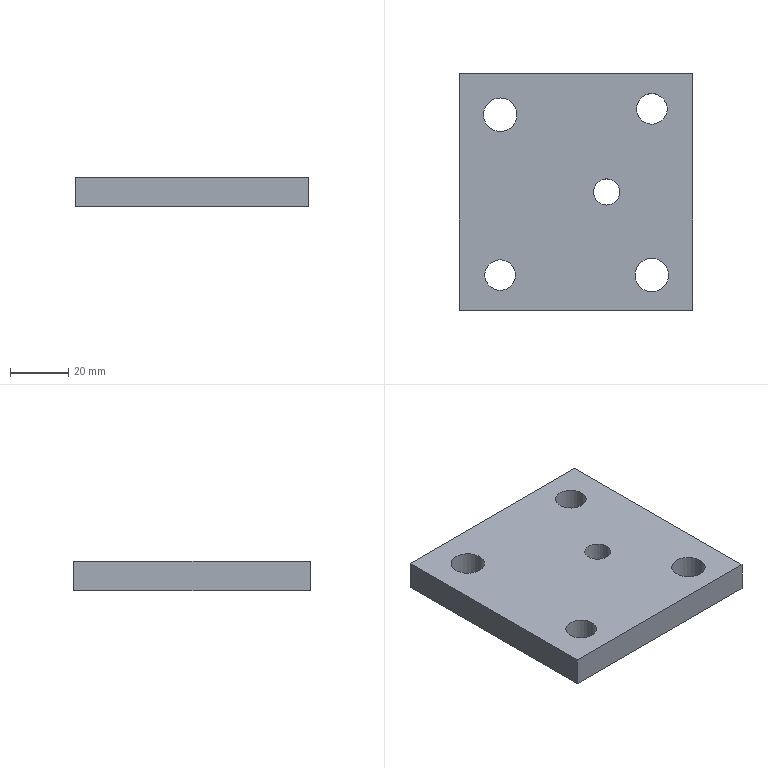Part | NX | features 6 2 | 1 solid | 11 faces | box 80 x 81 x 10 mm | volume 60355 mm3 | plane 6 | cylinder 5 | commonest cylinder face diameters 10.5 x2 11.5 x2 9 x1
STEP:
#1=CARTESIAN_POINT('',(3424.438,82.438,101.));
#2=VERTEX_POINT('',#1);
#3=CARTESIAN_POINT('',(3424.438,1.438,101.));
#4=VERTEX_POINT('',#3);
#5=CARTESIAN_POINT('',(3424.438,41.938,101.));
#6=DIRECTION('',(0.,-1.,0.));
#7=VECTOR('',#6,1000.);
#8=LINE('',#5,#7);
#9=EDGE_CURVE('',#2,#4,#8,.T.);
#10=ORIENTED_EDGE('',*,*,#9,.T.);
#11=CARTESIAN_POINT('',(3424.438,1.438,91.));
#12=VERTEX_POINT('',#11);
#13=CARTESIAN_POINT('',(3424.438,1.438,91.));
#14=DIRECTION('',(0.,0.,1.));
#15=VECTOR('',#14,1000.);
#16=LINE('',#13,#15);
#17=EDGE_CURVE('',#12,#4,#16,.T.);
#18=ORIENTED_EDGE('',*,*,#17,.F.);
#19=CARTESIAN_POINT('',(3424.438,82.438,91.));
#20=VERTEX_POINT('',#19);
#21=CARTESIAN_POINT('',(3424.438,41.938,91.));
#22=DIRECTION('',(0.,-1.,0.));
#23=VECTOR('',#22,1000.);
#24=LINE('',#21,#23);
#25=EDGE_CURVE('',#20,#12,#24,.T.);
#26=ORIENTED_EDGE('',*,*,#25,.F.);
#27=CARTESIAN_POINT('',(3424.438,82.438,91.));
#28=DIRECTION('',(0.,0.,-1.));
#29=VECTOR('',#28,1000.);
#30=LINE('',#27,#29);
#31=EDGE_CURVE('',#2,#20,#30,.T.);
#32=ORIENTED_EDGE('',*,*,#31,.F.);
#33=EDGE_LOOP('',(#10,#18,#26,#32));
#34=FACE_BOUND('',#33,.T.);
#35=CARTESIAN_POINT('',(3424.438,41.938,91.));
#36=DIRECTION('',(-1.,0.,0.));
#37=DIRECTION('',(0.,-1.,0.));
#38=AXIS2_PLACEMENT_3D('',#35,#36,#37);
#39=PLANE('',#38);
#40=ADVANCED_FACE('',(#34),#39,.F.);
#41=CARTESIAN_POINT('',(3344.438,82.438,101.));
#42=VERTEX_POINT('',#41);
#43=CARTESIAN_POINT('',(3374.438,82.438,101.));
#44=DIRECTION('',(1.,0.,0.));
#45=VECTOR('',#44,1000.);
#46=LINE('',#43,#45);
#47=EDGE_CURVE('',#42,#2,#46,.T.);
#48=ORIENTED_EDGE('',*,*,#47,.T.);
#49=ORIENTED_EDGE('',*,*,#31,.T.);
#50=CARTESIAN_POINT('',(3344.438,82.438,91.));
#51=VERTEX_POINT('',#50);
#52=CARTESIAN_POINT('',(3374.438,82.438,91.));
#53=DIRECTION('',(1.,0.,0.));
#54=VECTOR('',#53,1000.);
#55=LINE('',#52,#54);
#56=EDGE_CURVE('',#51,#20,#55,.T.);
#57=ORIENTED_EDGE('',*,*,#56,.F.);
#58=CARTESIAN_POINT('',(3344.438,82.438,91.));
#59=DIRECTION('',(0.,0.,-1.));
#60=VECTOR('',#59,1000.);
#61=LINE('',#58,#60);
#62=EDGE_CURVE('',#42,#51,#61,.T.);
#63=ORIENTED_EDGE('',*,*,#62,.F.);
#64=EDGE_LOOP('',(#48,#49,#57,#63));
#65=FACE_BOUND('',#64,.T.);
#66=CARTESIAN_POINT('',(3374.438,82.438,91.));
#67=DIRECTION('',(0.,-1.,0.));
#68=DIRECTION('',(1.,0.,0.));
#69=AXIS2_PLACEMENT_3D('',#66,#67,#68);
#70=PLANE('',#69);
#71=ADVANCED_FACE('',(#65),#70,.F.);
#72=CARTESIAN_POINT('',(3344.438,1.438,101.));
#73=VERTEX_POINT('',#72);
#74=CARTESIAN_POINT('',(3344.438,41.938,101.));
#75=DIRECTION('',(0.,1.,0.));
#76=VECTOR('',#75,1000.);
#77=LINE('',#74,#76);
#78=EDGE_CURVE('',#73,#42,#77,.T.);
#79=ORIENTED_EDGE('',*,*,#78,.T.);
#80=ORIENTED_EDGE('',*,*,#62,.T.);
#81=CARTESIAN_POINT('',(3344.438,1.438,91.));
#82=VERTEX_POINT('',#81);
#83=CARTESIAN_POINT('',(3344.438,41.938,91.));
#84=DIRECTION('',(0.,1.,0.));
#85=VECTOR('',#84,1000.);
#86=LINE('',#83,#85);
#87=EDGE_CURVE('',#82,#51,#86,.T.);
#88=ORIENTED_EDGE('',*,*,#87,.F.);
#89=CARTESIAN_POINT('',(3344.438,1.438,91.));
#90=DIRECTION('',(0.,0.,-1.));
#91=VECTOR('',#90,1000.);
#92=LINE('',#89,#91);
#93=EDGE_CURVE('',#73,#82,#92,.T.);
#94=ORIENTED_EDGE('',*,*,#93,.F.);
#95=EDGE_LOOP('',(#79,#80,#88,#94));
#96=FACE_BOUND('',#95,.T.);
#97=CARTESIAN_POINT('',(3344.438,41.938,91.));
#98=DIRECTION('',(1.,0.,0.));
#99=DIRECTION('',(0.,1.,0.));
#100=AXIS2_PLACEMENT_3D('',#97,#98,#99);
#101=PLANE('',#100);
#102=ADVANCED_FACE('',(#96),#101,.F.);
#103=CARTESIAN_POINT('',(3358.438,8.188,91.));
#104=VERTEX_POINT('',#103);
#105=CARTESIAN_POINT('',(3358.438,13.438,91.));
#106=DIRECTION('',(0.,0.,-1.));
#107=DIRECTION('',(0.,-1.,0.));
#108=AXIS2_PLACEMENT_3D('',#105,#106,#107);
#109=CIRCLE('',#108,5.25);
#110=EDGE_CURVE('',#104,#104,#109,.T.);
#111=ORIENTED_EDGE('',*,*,#110,.T.);
#112=EDGE_LOOP('',(#111));
#113=FACE_BOUND('',#112,.T.);
#114=CARTESIAN_POINT('',(3358.438,18.688,101.));
#115=VERTEX_POINT('',#114);
#116=CARTESIAN_POINT('',(3358.438,13.438,101.));
#117=DIRECTION('',(0.,0.,1.));
#118=DIRECTION('',(0.,1.,0.));
#119=AXIS2_PLACEMENT_3D('',#116,#117,#118);
#120=CIRCLE('',#119,5.25);
#121=EDGE_CURVE('',#115,#115,#120,.T.);
#122=ORIENTED_EDGE('',*,*,#121,.T.);
#123=EDGE_LOOP('',(#122));
#124=FACE_BOUND('',#123,.T.);
#125=CARTESIAN_POINT('',(3358.438,13.438,91.));
#126=DIRECTION('',(0.,0.,1.));
#127=DIRECTION('',(0.,-1.,0.));
#128=AXIS2_PLACEMENT_3D('',#125,#126,#127);
#129=CYLINDRICAL_SURFACE('',#128,5.25);
#130=ADVANCED_FACE('',(#113,#124),#129,.F.);
#131=CARTESIAN_POINT('',(3410.438,19.188,91.));
#132=VERTEX_POINT('',#131);
#133=CARTESIAN_POINT('',(3410.438,13.438,91.));
#134=DIRECTION('',(0.,0.,1.));
#135=DIRECTION('',(0.,1.,0.));
#136=AXIS2_PLACEMENT_3D('',#133,#134,#135);
#137=CIRCLE('',#136,5.75);
#138=EDGE_CURVE('',#132,#132,#137,.T.);
#139=ORIENTED_EDGE('',*,*,#138,.F.);
#140=EDGE_LOOP('',(#139));
#141=FACE_BOUND('',#140,.T.);
#142=CARTESIAN_POINT('',(3410.438,19.188,101.));
#143=VERTEX_POINT('',#142);
#144=CARTESIAN_POINT('',(3410.438,13.438,101.));
#145=DIRECTION('',(0.,0.,1.));
#146=DIRECTION('',(0.,1.,0.));
#147=AXIS2_PLACEMENT_3D('',#144,#145,#146);
#148=CIRCLE('',#147,5.75);
#149=EDGE_CURVE('',#143,#143,#148,.T.);
#150=ORIENTED_EDGE('',*,*,#149,.T.);
#151=EDGE_LOOP('',(#150));
#152=FACE_BOUND('',#151,.T.);
#153=CARTESIAN_POINT('',(3410.438,13.438,91.));
#154=DIRECTION('',(0.,0.,1.));
#155=DIRECTION('',(0.,-1.,0.));
#156=AXIS2_PLACEMENT_3D('',#153,#154,#155);
#157=CYLINDRICAL_SURFACE('',#156,5.75);
#158=ADVANCED_FACE('',(#141,#152),#157,.F.);
#159=CARTESIAN_POINT('',(3374.438,1.438,91.));
#160=DIRECTION('',(-1.,0.,0.));
#161=VECTOR('',#160,1000.);
#162=LINE('',#159,#161);
#163=EDGE_CURVE('',#12,#82,#162,.T.);
#164=ORIENTED_EDGE('',*,*,#163,.F.);
#165=ORIENTED_EDGE('',*,*,#17,.T.);
#166=CARTESIAN_POINT('',(3374.438,1.438,101.));
#167=DIRECTION('',(-1.,0.,0.));
#168=VECTOR('',#167,1000.);
#169=LINE('',#166,#168);
#170=EDGE_CURVE('',#4,#73,#169,.T.);
#171=ORIENTED_EDGE('',*,*,#170,.T.);
#172=ORIENTED_EDGE('',*,*,#93,.T.);
#173=EDGE_LOOP('',(#164,#165,#171,#172));
#174=FACE_BOUND('',#173,.T.);
#175=CARTESIAN_POINT('',(3374.438,1.438,91.));
#176=DIRECTION('',(0.,1.,0.));
#177=DIRECTION('',(-1.,0.,0.));
#178=AXIS2_PLACEMENT_3D('',#175,#176,#177);
#179=PLANE('',#178);
#180=ADVANCED_FACE('',(#174),#179,.F.);
#181=CARTESIAN_POINT('',(3358.438,74.188,91.));
#182=VERTEX_POINT('',#181);
#183=CARTESIAN_POINT('',(3358.438,68.438,91.));
#184=DIRECTION('',(0.,0.,1.));
#185=DIRECTION('',(0.,1.,0.));
#186=AXIS2_PLACEMENT_3D('',#183,#184,#185);
#187=CIRCLE('',#186,5.75);
#188=EDGE_CURVE('',#182,#182,#187,.T.);
#189=ORIENTED_EDGE('',*,*,#188,.F.);
#190=EDGE_LOOP('',(#189));
#191=FACE_BOUND('',#190,.T.);
#192=CARTESIAN_POINT('',(3358.438,74.188,101.));
#193=VERTEX_POINT('',#192);
#194=CARTESIAN_POINT('',(3358.438,68.438,101.));
#195=DIRECTION('',(0.,0.,1.));
#196=DIRECTION('',(0.,1.,0.));
#197=AXIS2_PLACEMENT_3D('',#194,#195,#196);
#198=CIRCLE('',#197,5.75);
#199=EDGE_CURVE('',#193,#193,#198,.T.);
#200=ORIENTED_EDGE('',*,*,#199,.T.);
#201=EDGE_LOOP('',(#200));
#202=FACE_BOUND('',#201,.T.);
#203=CARTESIAN_POINT('',(3358.438,68.438,91.));
#204=DIRECTION('',(0.,0.,1.));
#205=DIRECTION('',(0.,-1.,0.));
#206=AXIS2_PLACEMENT_3D('',#203,#204,#205);
#207=CYLINDRICAL_SURFACE('',#206,5.75);
#208=ADVANCED_FACE('',(#191,#202),#207,.F.);
#209=CARTESIAN_POINT('',(3410.438,65.188,91.));
#210=VERTEX_POINT('',#209);
#211=CARTESIAN_POINT('',(3410.438,70.438,91.));
#212=DIRECTION('',(0.,0.,-1.));
#213=DIRECTION('',(0.,-1.,0.));
#214=AXIS2_PLACEMENT_3D('',#211,#212,#213);
#215=CIRCLE('',#214,5.25);
#216=EDGE_CURVE('',#210,#210,#215,.T.);
#217=ORIENTED_EDGE('',*,*,#216,.T.);
#218=EDGE_LOOP('',(#217));
#219=FACE_BOUND('',#218,.T.);
#220=CARTESIAN_POINT('',(3410.438,75.688,101.));
#221=VERTEX_POINT('',#220);
#222=CARTESIAN_POINT('',(3410.438,70.438,101.));
#223=DIRECTION('',(0.,0.,1.));
#224=DIRECTION('',(0.,1.,0.));
#225=AXIS2_PLACEMENT_3D('',#222,#223,#224);
#226=CIRCLE('',#225,5.25);
#227=EDGE_CURVE('',#221,#221,#226,.T.);
#228=ORIENTED_EDGE('',*,*,#227,.T.);
#229=EDGE_LOOP('',(#228));
#230=FACE_BOUND('',#229,.T.);
#231=CARTESIAN_POINT('',(3410.438,70.438,91.));
#232=DIRECTION('',(0.,0.,1.));
#233=DIRECTION('',(0.,-1.,0.));
#234=AXIS2_PLACEMENT_3D('',#231,#232,#233);
#235=CYLINDRICAL_SURFACE('',#234,5.25);
#236=ADVANCED_FACE('',(#219,#230),#235,.F.);
#237=CARTESIAN_POINT('',(3394.938,46.438,91.));
#238=VERTEX_POINT('',#237);
#239=CARTESIAN_POINT('',(3394.938,41.938,91.));
#240=DIRECTION('',(0.,0.,-1.));
#241=DIRECTION('',(0.,1.,0.));
#242=AXIS2_PLACEMENT_3D('',#239,#240,#241);
#243=CIRCLE('',#242,4.5);
#244=EDGE_CURVE('',#238,#238,#243,.T.);
#245=ORIENTED_EDGE('',*,*,#244,.T.);
#246=EDGE_LOOP('',(#245));
#247=FACE_BOUND('',#246,.T.);
#248=CARTESIAN_POINT('',(3394.938,46.438,101.));
#249=VERTEX_POINT('',#248);
#250=CARTESIAN_POINT('',(3394.938,41.938,101.));
#251=DIRECTION('',(0.,0.,1.));
#252=DIRECTION('',(0.,1.,0.));
#253=AXIS2_PLACEMENT_3D('',#250,#251,#252);
#254=CIRCLE('',#253,4.5);
#255=EDGE_CURVE('',#249,#249,#254,.T.);
#256=ORIENTED_EDGE('',*,*,#255,.T.);
#257=EDGE_LOOP('',(#256));
#258=FACE_BOUND('',#257,.T.);
#259=CARTESIAN_POINT('',(3394.938,41.938,-119.));
#260=DIRECTION('',(0.,0.,1.));
#261=DIRECTION('',(0.,-1.,0.));
#262=AXIS2_PLACEMENT_3D('',#259,#260,#261);
#263=CYLINDRICAL_SURFACE('',#262,4.5);
#264=ADVANCED_FACE('',(#247,#258),#263,.F.);
#265=ORIENTED_EDGE('',*,*,#216,.F.);
#266=EDGE_LOOP('',(#265));
#267=FACE_BOUND('',#266,.T.);
#268=ORIENTED_EDGE('',*,*,#188,.T.);
#269=EDGE_LOOP('',(#268));
#270=FACE_BOUND('',#269,.T.);
#271=ORIENTED_EDGE('',*,*,#87,.T.);
#272=ORIENTED_EDGE('',*,*,#56,.T.);
#273=ORIENTED_EDGE('',*,*,#25,.T.);
#274=ORIENTED_EDGE('',*,*,#163,.T.);
#275=EDGE_LOOP('',(#271,#272,#273,#274));
#276=FACE_BOUND('',#275,.T.);
#277=ORIENTED_EDGE('',*,*,#138,.T.);
#278=EDGE_LOOP('',(#277));
#279=FACE_BOUND('',#278,.T.);
#280=ORIENTED_EDGE('',*,*,#110,.F.);
#281=EDGE_LOOP('',(#280));
#282=FACE_BOUND('',#281,.T.);
#283=ORIENTED_EDGE('',*,*,#244,.F.);
#284=EDGE_LOOP('',(#283));
#285=FACE_BOUND('',#284,.T.);
#286=CARTESIAN_POINT('',(3374.438,41.938,91.));
#287=DIRECTION('',(0.,0.,1.));
#288=DIRECTION('',(0.,-1.,0.));
#289=AXIS2_PLACEMENT_3D('',#286,#287,#288);
#290=PLANE('',#289);
#291=ADVANCED_FACE('',(#267,#270,#276,#279,#282,#285),#290,.F.);
#292=ORIENTED_EDGE('',*,*,#121,.F.);
#293=EDGE_LOOP('',(#292));
#294=FACE_BOUND('',#293,.T.);
#295=ORIENTED_EDGE('',*,*,#149,.F.);
#296=EDGE_LOOP('',(#295));
#297=FACE_BOUND('',#296,.T.);
#298=ORIENTED_EDGE('',*,*,#170,.F.);
#299=ORIENTED_EDGE('',*,*,#9,.F.);
#300=ORIENTED_EDGE('',*,*,#47,.F.);
#301=ORIENTED_EDGE('',*,*,#78,.F.);
#302=EDGE_LOOP('',(#298,#299,#300,#301));
#303=FACE_BOUND('',#302,.T.);
#304=ORIENTED_EDGE('',*,*,#199,.F.);
#305=EDGE_LOOP('',(#304));
#306=FACE_BOUND('',#305,.T.);
#307=ORIENTED_EDGE('',*,*,#227,.F.);
#308=EDGE_LOOP('',(#307));
#309=FACE_BOUND('',#308,.T.);
#310=ORIENTED_EDGE('',*,*,#255,.F.);
#311=EDGE_LOOP('',(#310));
#312=FACE_BOUND('',#311,.T.);
#313=CARTESIAN_POINT('',(3556.438,1171.938,101.));
#314=DIRECTION('',(0.,0.,1.));
#315=DIRECTION('',(0.,1.,0.));
#316=AXIS2_PLACEMENT_3D('',#313,#314,#315);
#317=PLANE('',#316);
#318=ADVANCED_FACE('',(#294,#297,#303,#306,#309,#312),#317,.T.);
#319=CLOSED_SHELL('',(#40,#71,#102,#130,#158,#180,#208,#236,#264,#291,#318));
#320=MANIFOLD_SOLID_BREP('',#319);
#321=(LENGTH_UNIT()NAMED_UNIT(*)SI_UNIT(.MILLI.,.METRE.));
#322=UNCERTAINTY_MEASURE_WITH_UNIT(LENGTH_MEASURE(0.00001),#321,'','');
#323=(NAMED_UNIT(*)PLANE_ANGLE_UNIT()SI_UNIT($,.RADIAN.));
#324=(NAMED_UNIT(*)SI_UNIT($,.STERADIAN.)SOLID_ANGLE_UNIT());
#325=(GEOMETRIC_REPRESENTATION_CONTEXT(3)GLOBAL_UNCERTAINTY_ASSIGNED_CONTEXT((#322))GLOBAL_UNIT_ASSIGNED_CONTEXT((#321,#323,#324))REPRESENTATION_CONTEXT('',''));
#326=ADVANCED_BREP_SHAPE_REPRESENTATION('',(#320),#325);